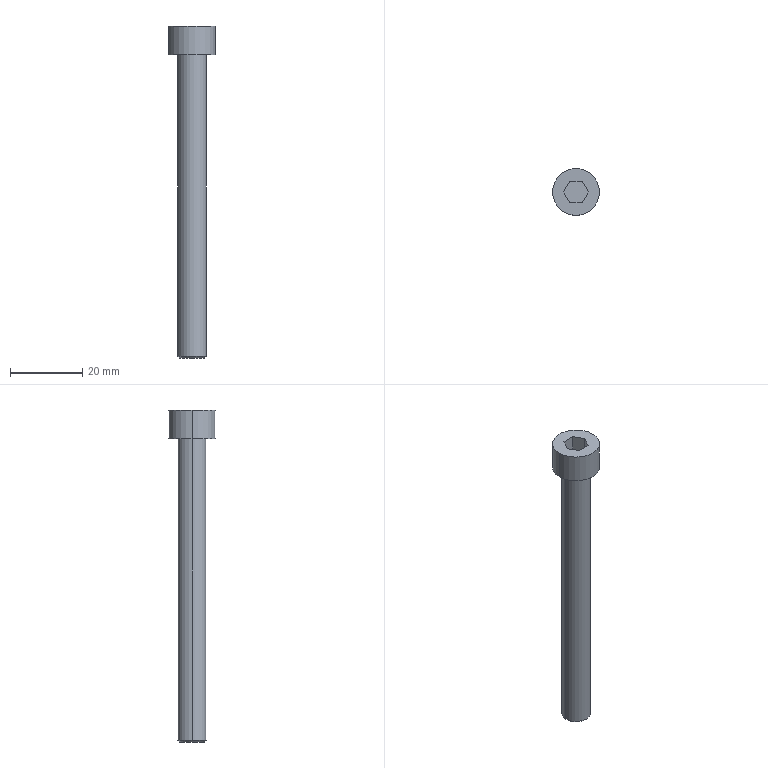Part | Creo | 1 solid | 16 faces | box 13 x 13 x 92 mm | volume 5116 mm3 | plane 10 | cylinder 4 | cone 2 | commonest cylinder face diameters 8 x2 13 x2
STEP:
#1=CARTESIAN_POINT('',(0.,0.,0.));
#2=DIRECTION('',(0.,0.,1.));
#3=DIRECTION('',(1.,0.,0.));
#4=AXIS2_PLACEMENT_3D('',#1,#2,#3);
#5=CARTESIAN_POINT('',(464.154,190.125,-122.934));
#6=VERTEX_POINT('',#5);
#7=CARTESIAN_POINT('',(472.154,190.125,-122.934));
#8=VERTEX_POINT('',#7);
#9=CARTESIAN_POINT('',(468.154,190.125,-122.934));
#10=DIRECTION('',(0.,0.,-1.));
#11=DIRECTION('',(-1.,0.,0.));
#12=AXIS2_PLACEMENT_3D('',#9,#10,#11);
#13=CIRCLE('',#12,4.);
#14=EDGE_CURVE('',#6,#8,#13,.T.);
#15=ORIENTED_EDGE('',*,*,#14,.T.);
#16=CARTESIAN_POINT('',(472.154,190.125,-39.441));
#17=VERTEX_POINT('',#16);
#18=CARTESIAN_POINT('',(472.154,190.125,-39.441));
#19=DIRECTION('',(0.,0.,-1.));
#20=VECTOR('',#19,83.493);
#21=LINE('',#18,#20);
#22=EDGE_CURVE('',#17,#8,#21,.T.);
#23=ORIENTED_EDGE('',*,*,#22,.F.);
#24=CARTESIAN_POINT('',(464.154,190.125,-39.441));
#25=VERTEX_POINT('',#24);
#26=CARTESIAN_POINT('',(468.154,190.125,-39.441));
#27=DIRECTION('',(0.,0.,1.));
#28=DIRECTION('',(1.,0.,0.));
#29=AXIS2_PLACEMENT_3D('',#26,#27,#28);
#30=CIRCLE('',#29,4.);
#31=EDGE_CURVE('',#17,#25,#30,.T.);
#32=ORIENTED_EDGE('',*,*,#31,.T.);
#33=CARTESIAN_POINT('',(464.154,190.125,-39.441));
#34=DIRECTION('',(0.,0.,-1.));
#35=VECTOR('',#34,83.493);
#36=LINE('',#33,#35);
#37=EDGE_CURVE('',#25,#6,#36,.T.);
#38=ORIENTED_EDGE('',*,*,#37,.T.);
#39=EDGE_LOOP('',(#15,#23,#32,#38));
#40=FACE_OUTER_BOUND('',#39,.F.);
#41=CARTESIAN_POINT('',(468.154,190.125,-39.441));
#42=DIRECTION('',(0.,0.,-1.));
#43=DIRECTION('',(-1.,0.,0.));
#44=AXIS2_PLACEMENT_3D('',#41,#42,#43);
#45=CYLINDRICAL_SURFACE('',#44,4.);
#46=ADVANCED_FACE('',(#40),#45,.T.);
#47=CARTESIAN_POINT('',(464.662,190.125,-123.441));
#48=VERTEX_POINT('',#47);
#49=CARTESIAN_POINT('',(471.647,190.125,-123.441));
#50=VERTEX_POINT('',#49);
#51=CARTESIAN_POINT('',(468.154,190.125,-123.441));
#52=DIRECTION('',(0.,0.,-1.));
#53=DIRECTION('',(-1.,0.,0.));
#54=AXIS2_PLACEMENT_3D('',#51,#52,#53);
#55=CIRCLE('',#54,3.493);
#56=EDGE_CURVE('',#48,#50,#55,.T.);
#57=ORIENTED_EDGE('',*,*,#56,.T.);
#58=CARTESIAN_POINT('',(471.647,190.125,-123.441));
#59=DIRECTION('',(0.7071,0.,0.7071));
#60=VECTOR('',#59,0.7176);
#61=LINE('',#58,#60);
#62=EDGE_CURVE('',#50,#8,#61,.T.);
#63=ORIENTED_EDGE('',*,*,#62,.T.);
#64=ORIENTED_EDGE('',*,*,#14,.F.);
#65=CARTESIAN_POINT('',(464.662,190.125,-123.441));
#66=DIRECTION('',(-0.7071,0.,0.7071));
#67=VECTOR('',#66,0.7176);
#68=LINE('',#65,#67);
#69=EDGE_CURVE('',#48,#6,#68,.T.);
#70=ORIENTED_EDGE('',*,*,#69,.F.);
#71=EDGE_LOOP('',(#57,#63,#64,#70));
#72=FACE_OUTER_BOUND('',#71,.F.);
#73=CARTESIAN_POINT('',(468.154,190.125,-123.188));
#74=DIRECTION('',(0.,0.,1.));
#75=DIRECTION('',(1.,0.,0.));
#76=AXIS2_PLACEMENT_3D('',#73,#74,#75);
#77=CONICAL_SURFACE('',#76,3.746,45.);
#78=ADVANCED_FACE('',(#72),#77,.T.);
#79=ORIENTED_EDGE('',*,*,#56,.F.);
#80=CARTESIAN_POINT('',(468.154,190.125,-123.441));
#81=DIRECTION('',(0.,0.,-1.));
#82=DIRECTION('',(1.,0.,0.));
#83=AXIS2_PLACEMENT_3D('',#80,#81,#82);
#84=CIRCLE('',#83,3.493);
#85=EDGE_CURVE('',#50,#48,#84,.T.);
#86=ORIENTED_EDGE('',*,*,#85,.F.);
#87=EDGE_LOOP('',(#79,#86));
#88=FACE_OUTER_BOUND('',#87,.F.);
#89=CARTESIAN_POINT('',(468.154,190.125,-123.441));
#90=DIRECTION('',(0.,0.,1.));
#91=DIRECTION('',(1.,0.,0.));
#92=AXIS2_PLACEMENT_3D('',#89,#90,#91);
#93=PLANE('',#92);
#94=ADVANCED_FACE('',(#88),#93,.F.);
#95=ORIENTED_EDGE('',*,*,#85,.T.);
#96=ORIENTED_EDGE('',*,*,#69,.T.);
#97=CARTESIAN_POINT('',(468.154,190.125,-122.934));
#98=DIRECTION('',(0.,0.,-1.));
#99=DIRECTION('',(1.,0.,0.));
#100=AXIS2_PLACEMENT_3D('',#97,#98,#99);
#101=CIRCLE('',#100,4.);
#102=EDGE_CURVE('',#8,#6,#101,.T.);
#103=ORIENTED_EDGE('',*,*,#102,.F.);
#104=ORIENTED_EDGE('',*,*,#62,.F.);
#105=EDGE_LOOP('',(#95,#96,#103,#104));
#106=FACE_OUTER_BOUND('',#105,.F.);
#107=CARTESIAN_POINT('',(468.154,190.125,-123.188));
#108=DIRECTION('',(0.,0.,1.));
#109=DIRECTION('',(1.,0.,0.));
#110=AXIS2_PLACEMENT_3D('',#107,#108,#109);
#111=CONICAL_SURFACE('',#110,3.746,45.);
#112=ADVANCED_FACE('',(#106),#111,.T.);
#113=ORIENTED_EDGE('',*,*,#102,.T.);
#114=ORIENTED_EDGE('',*,*,#37,.F.);
#115=CARTESIAN_POINT('',(468.154,190.125,-39.441));
#116=DIRECTION('',(0.,0.,1.));
#117=DIRECTION('',(-1.,0.,0.));
#118=AXIS2_PLACEMENT_3D('',#115,#116,#117);
#119=CIRCLE('',#118,4.);
#120=EDGE_CURVE('',#25,#17,#119,.T.);
#121=ORIENTED_EDGE('',*,*,#120,.T.);
#122=ORIENTED_EDGE('',*,*,#22,.T.);
#123=EDGE_LOOP('',(#113,#114,#121,#122));
#124=FACE_OUTER_BOUND('',#123,.F.);
#125=CARTESIAN_POINT('',(468.154,190.125,-39.441));
#126=DIRECTION('',(0.,0.,-1.));
#127=DIRECTION('',(-1.,0.,0.));
#128=AXIS2_PLACEMENT_3D('',#125,#126,#127);
#129=CYLINDRICAL_SURFACE('',#128,4.);
#130=ADVANCED_FACE('',(#124),#129,.T.);
#131=CARTESIAN_POINT('',(461.654,190.125,-39.441));
#132=VERTEX_POINT('',#131);
#133=CARTESIAN_POINT('',(474.654,190.125,-39.441));
#134=VERTEX_POINT('',#133);
#135=CARTESIAN_POINT('',(468.154,190.125,-39.441));
#136=DIRECTION('',(0.,0.,-1.));
#137=DIRECTION('',(-1.,0.,0.));
#138=AXIS2_PLACEMENT_3D('',#135,#136,#137);
#139=CIRCLE('',#138,6.5);
#140=EDGE_CURVE('',#132,#134,#139,.T.);
#141=ORIENTED_EDGE('',*,*,#140,.F.);
#142=CARTESIAN_POINT('',(468.154,190.125,-39.441));
#143=DIRECTION('',(0.,0.,-1.));
#144=DIRECTION('',(1.,0.,0.));
#145=AXIS2_PLACEMENT_3D('',#142,#143,#144);
#146=CIRCLE('',#145,6.5);
#147=EDGE_CURVE('',#134,#132,#146,.T.);
#148=ORIENTED_EDGE('',*,*,#147,.F.);
#149=EDGE_LOOP('',(#141,#148));
#150=FACE_OUTER_BOUND('',#149,.F.);
#151=ORIENTED_EDGE('',*,*,#120,.F.);
#152=ORIENTED_EDGE('',*,*,#31,.F.);
#153=EDGE_LOOP('',(#151,#152));
#154=FACE_BOUND('',#153,.F.);
#155=CARTESIAN_POINT('',(468.154,190.125,-39.441));
#156=DIRECTION('',(0.,0.,-1.));
#157=DIRECTION('',(-1.,0.,0.));
#158=AXIS2_PLACEMENT_3D('',#155,#156,#157);
#159=PLANE('',#158);
#160=ADVANCED_FACE('',(#150,#154),#159,.T.);
#161=CARTESIAN_POINT('',(474.654,190.125,-31.441));
#162=VERTEX_POINT('',#161);
#163=CARTESIAN_POINT('',(461.654,190.125,-31.441));
#164=VERTEX_POINT('',#163);
#165=CARTESIAN_POINT('',(468.154,190.125,-31.441));
#166=DIRECTION('',(0.,0.,1.));
#167=DIRECTION('',(1.,0.,0.));
#168=AXIS2_PLACEMENT_3D('',#165,#166,#167);
#169=CIRCLE('',#168,6.5);
#170=EDGE_CURVE('',#162,#164,#169,.T.);
#171=ORIENTED_EDGE('',*,*,#170,.T.);
#172=CARTESIAN_POINT('',(461.654,190.125,-39.441));
#173=DIRECTION('',(0.,0.,1.));
#174=VECTOR('',#173,8.);
#175=LINE('',#172,#174);
#176=EDGE_CURVE('',#132,#164,#175,.T.);
#177=ORIENTED_EDGE('',*,*,#176,.F.);
#178=ORIENTED_EDGE('',*,*,#140,.T.);
#179=CARTESIAN_POINT('',(474.654,190.125,-39.441));
#180=DIRECTION('',(0.,0.,1.));
#181=VECTOR('',#180,8.);
#182=LINE('',#179,#181);
#183=EDGE_CURVE('',#134,#162,#182,.T.);
#184=ORIENTED_EDGE('',*,*,#183,.T.);
#185=EDGE_LOOP('',(#171,#177,#178,#184));
#186=FACE_OUTER_BOUND('',#185,.F.);
#187=CARTESIAN_POINT('',(468.154,190.125,-39.441));
#188=DIRECTION('',(0.,0.,1.));
#189=DIRECTION('',(1.,0.,0.));
#190=AXIS2_PLACEMENT_3D('',#187,#188,#189);
#191=CYLINDRICAL_SURFACE('',#190,6.5);
#192=ADVANCED_FACE('',(#186),#191,.T.);
#193=CARTESIAN_POINT('',(468.154,190.125,-31.441));
#194=DIRECTION('',(0.,0.,1.));
#195=DIRECTION('',(-1.,0.,0.));
#196=AXIS2_PLACEMENT_3D('',#193,#194,#195);
#197=CIRCLE('',#196,6.5);
#198=EDGE_CURVE('',#164,#162,#197,.T.);
#199=ORIENTED_EDGE('',*,*,#198,.F.);
#200=ORIENTED_EDGE('',*,*,#170,.F.);
#201=EDGE_LOOP('',(#199,#200));
#202=FACE_OUTER_BOUND('',#201,.F.);
#203=CARTESIAN_POINT('',(466.422,193.125,-31.441));
#204=VERTEX_POINT('',#203);
#205=CARTESIAN_POINT('',(469.886,193.125,-31.441));
#206=VERTEX_POINT('',#205);
#207=CARTESIAN_POINT('',(466.422,193.125,-31.441));
#208=DIRECTION('',(1.,0.,0.));
#209=VECTOR('',#208,3.464);
#210=LINE('',#207,#209);
#211=EDGE_CURVE('',#204,#206,#210,.T.);
#212=ORIENTED_EDGE('',*,*,#211,.F.);
#213=CARTESIAN_POINT('',(464.69,190.125,-31.441));
#214=VERTEX_POINT('',#213);
#215=CARTESIAN_POINT('',(464.69,190.125,-31.441));
#216=DIRECTION('',(0.5,0.866,0.));
#217=VECTOR('',#216,3.464);
#218=LINE('',#215,#217);
#219=EDGE_CURVE('',#214,#204,#218,.T.);
#220=ORIENTED_EDGE('',*,*,#219,.F.);
#221=CARTESIAN_POINT('',(466.422,187.125,-31.441));
#222=VERTEX_POINT('',#221);
#223=CARTESIAN_POINT('',(466.422,187.125,-31.441));
#224=DIRECTION('',(-0.5,0.866,0.));
#225=VECTOR('',#224,3.464);
#226=LINE('',#223,#225);
#227=EDGE_CURVE('',#222,#214,#226,.T.);
#228=ORIENTED_EDGE('',*,*,#227,.F.);
#229=CARTESIAN_POINT('',(469.886,187.125,-31.441));
#230=VERTEX_POINT('',#229);
#231=CARTESIAN_POINT('',(469.886,187.125,-31.441));
#232=DIRECTION('',(-1.,0.,0.));
#233=VECTOR('',#232,3.464);
#234=LINE('',#231,#233);
#235=EDGE_CURVE('',#230,#222,#234,.T.);
#236=ORIENTED_EDGE('',*,*,#235,.F.);
#237=CARTESIAN_POINT('',(471.618,190.125,-31.441));
#238=VERTEX_POINT('',#237);
#239=CARTESIAN_POINT('',(471.618,190.125,-31.441));
#240=DIRECTION('',(-0.5,-0.866,0.));
#241=VECTOR('',#240,3.464);
#242=LINE('',#239,#241);
#243=EDGE_CURVE('',#238,#230,#242,.T.);
#244=ORIENTED_EDGE('',*,*,#243,.F.);
#245=CARTESIAN_POINT('',(469.886,193.125,-31.441));
#246=DIRECTION('',(0.5,-0.866,0.));
#247=VECTOR('',#246,3.464);
#248=LINE('',#245,#247);
#249=EDGE_CURVE('',#206,#238,#248,.T.);
#250=ORIENTED_EDGE('',*,*,#249,.F.);
#251=EDGE_LOOP('',(#212,#220,#228,#236,#244,#250));
#252=FACE_BOUND('',#251,.F.);
#253=CARTESIAN_POINT('',(468.154,190.125,-31.441));
#254=DIRECTION('',(0.,0.,1.));
#255=DIRECTION('',(1.,0.,0.));
#256=AXIS2_PLACEMENT_3D('',#253,#254,#255);
#257=PLANE('',#256);
#258=ADVANCED_FACE('',(#202,#252),#257,.T.);
#259=ORIENTED_EDGE('',*,*,#211,.T.);
#260=CARTESIAN_POINT('',(469.886,193.125,-36.721));
#261=VERTEX_POINT('',#260);
#262=CARTESIAN_POINT('',(469.886,193.125,-31.441));
#263=DIRECTION('',(0.,0.,-1.));
#264=VECTOR('',#263,5.28);
#265=LINE('',#262,#264);
#266=EDGE_CURVE('',#206,#261,#265,.T.);
#267=ORIENTED_EDGE('',*,*,#266,.T.);
#268=CARTESIAN_POINT('',(466.422,193.125,-36.721));
#269=VERTEX_POINT('',#268);
#270=CARTESIAN_POINT('',(466.422,193.125,-36.721));
#271=DIRECTION('',(1.,0.,0.));
#272=VECTOR('',#271,3.464);
#273=LINE('',#270,#272);
#274=EDGE_CURVE('',#269,#261,#273,.T.);
#275=ORIENTED_EDGE('',*,*,#274,.F.);
#276=CARTESIAN_POINT('',(466.422,193.125,-31.441));
#277=DIRECTION('',(0.,0.,-1.));
#278=VECTOR('',#277,5.28);
#279=LINE('',#276,#278);
#280=EDGE_CURVE('',#204,#269,#279,.T.);
#281=ORIENTED_EDGE('',*,*,#280,.F.);
#282=EDGE_LOOP('',(#259,#267,#275,#281));
#283=FACE_OUTER_BOUND('',#282,.F.);
#284=CARTESIAN_POINT('',(469.886,193.125,-36.721));
#285=DIRECTION('',(0.,1.,0.));
#286=DIRECTION('',(0.,0.,1.));
#287=AXIS2_PLACEMENT_3D('',#284,#285,#286);
#288=PLANE('',#287);
#289=ADVANCED_FACE('',(#283),#288,.F.);
#290=ORIENTED_EDGE('',*,*,#249,.T.);
#291=CARTESIAN_POINT('',(471.618,190.125,-36.721));
#292=VERTEX_POINT('',#291);
#293=CARTESIAN_POINT('',(471.618,190.125,-31.441));
#294=DIRECTION('',(0.,0.,-1.));
#295=VECTOR('',#294,5.28);
#296=LINE('',#293,#295);
#297=EDGE_CURVE('',#238,#292,#296,.T.);
#298=ORIENTED_EDGE('',*,*,#297,.T.);
#299=CARTESIAN_POINT('',(471.618,190.125,-36.721));
#300=DIRECTION('',(-0.5,0.866,0.));
#301=VECTOR('',#300,3.464);
#302=LINE('',#299,#301);
#303=EDGE_CURVE('',#292,#261,#302,.T.);
#304=ORIENTED_EDGE('',*,*,#303,.T.);
#305=ORIENTED_EDGE('',*,*,#266,.F.);
#306=EDGE_LOOP('',(#290,#298,#304,#305));
#307=FACE_OUTER_BOUND('',#306,.F.);
#308=CARTESIAN_POINT('',(471.618,190.125,-36.721));
#309=DIRECTION('',(0.866,0.5,0.));
#310=DIRECTION('',(-0.5,0.866,0.));
#311=AXIS2_PLACEMENT_3D('',#308,#309,#310);
#312=PLANE('',#311);
#313=ADVANCED_FACE('',(#307),#312,.F.);
#314=ORIENTED_EDGE('',*,*,#243,.T.);
#315=CARTESIAN_POINT('',(469.886,187.125,-36.721));
#316=VERTEX_POINT('',#315);
#317=CARTESIAN_POINT('',(469.886,187.125,-31.441));
#318=DIRECTION('',(0.,0.,-1.));
#319=VECTOR('',#318,5.28);
#320=LINE('',#317,#319);
#321=EDGE_CURVE('',#230,#316,#320,.T.);
#322=ORIENTED_EDGE('',*,*,#321,.T.);
#323=CARTESIAN_POINT('',(469.886,187.125,-36.721));
#324=DIRECTION('',(0.5,0.866,0.));
#325=VECTOR('',#324,3.464);
#326=LINE('',#323,#325);
#327=EDGE_CURVE('',#316,#292,#326,.T.);
#328=ORIENTED_EDGE('',*,*,#327,.T.);
#329=ORIENTED_EDGE('',*,*,#297,.F.);
#330=EDGE_LOOP('',(#314,#322,#328,#329));
#331=FACE_OUTER_BOUND('',#330,.F.);
#332=CARTESIAN_POINT('',(469.886,187.125,-36.721));
#333=DIRECTION('',(0.866,-0.5,0.));
#334=DIRECTION('',(0.5,0.866,0.));
#335=AXIS2_PLACEMENT_3D('',#332,#333,#334);
#336=PLANE('',#335);
#337=ADVANCED_FACE('',(#331),#336,.F.);
#338=ORIENTED_EDGE('',*,*,#235,.T.);
#339=CARTESIAN_POINT('',(466.422,187.125,-36.721));
#340=VERTEX_POINT('',#339);
#341=CARTESIAN_POINT('',(466.422,187.125,-31.441));
#342=DIRECTION('',(0.,0.,-1.));
#343=VECTOR('',#342,5.28);
#344=LINE('',#341,#343);
#345=EDGE_CURVE('',#222,#340,#344,.T.);
#346=ORIENTED_EDGE('',*,*,#345,.T.);
#347=CARTESIAN_POINT('',(469.886,187.125,-36.721));
#348=DIRECTION('',(-1.,0.,0.));
#349=VECTOR('',#348,3.464);
#350=LINE('',#347,#349);
#351=EDGE_CURVE('',#316,#340,#350,.T.);
#352=ORIENTED_EDGE('',*,*,#351,.F.);
#353=ORIENTED_EDGE('',*,*,#321,.F.);
#354=EDGE_LOOP('',(#338,#346,#352,#353));
#355=FACE_OUTER_BOUND('',#354,.F.);
#356=CARTESIAN_POINT('',(466.422,187.125,-36.721));
#357=DIRECTION('',(0.,-1.,0.));
#358=DIRECTION('',(0.,0.,-1.));
#359=AXIS2_PLACEMENT_3D('',#356,#357,#358);
#360=PLANE('',#359);
#361=ADVANCED_FACE('',(#355),#360,.F.);
#362=ORIENTED_EDGE('',*,*,#227,.T.);
#363=CARTESIAN_POINT('',(464.69,190.125,-36.721));
#364=VERTEX_POINT('',#363);
#365=CARTESIAN_POINT('',(464.69,190.125,-31.441));
#366=DIRECTION('',(0.,0.,-1.));
#367=VECTOR('',#366,5.28);
#368=LINE('',#365,#367);
#369=EDGE_CURVE('',#214,#364,#368,.T.);
#370=ORIENTED_EDGE('',*,*,#369,.T.);
#371=CARTESIAN_POINT('',(464.69,190.125,-36.721));
#372=DIRECTION('',(0.5,-0.866,0.));
#373=VECTOR('',#372,3.464);
#374=LINE('',#371,#373);
#375=EDGE_CURVE('',#364,#340,#374,.T.);
#376=ORIENTED_EDGE('',*,*,#375,.T.);
#377=ORIENTED_EDGE('',*,*,#345,.F.);
#378=EDGE_LOOP('',(#362,#370,#376,#377));
#379=FACE_OUTER_BOUND('',#378,.F.);
#380=CARTESIAN_POINT('',(464.69,190.125,-36.721));
#381=DIRECTION('',(-0.866,-0.5,0.));
#382=DIRECTION('',(0.5,-0.866,0.));
#383=AXIS2_PLACEMENT_3D('',#380,#381,#382);
#384=PLANE('',#383);
#385=ADVANCED_FACE('',(#379),#384,.F.);
#386=ORIENTED_EDGE('',*,*,#219,.T.);
#387=ORIENTED_EDGE('',*,*,#280,.T.);
#388=CARTESIAN_POINT('',(466.422,193.125,-36.721));
#389=DIRECTION('',(-0.5,-0.866,0.));
#390=VECTOR('',#389,3.464);
#391=LINE('',#388,#390);
#392=EDGE_CURVE('',#269,#364,#391,.T.);
#393=ORIENTED_EDGE('',*,*,#392,.T.);
#394=ORIENTED_EDGE('',*,*,#369,.F.);
#395=EDGE_LOOP('',(#386,#387,#393,#394));
#396=FACE_OUTER_BOUND('',#395,.F.);
#397=CARTESIAN_POINT('',(466.422,193.125,-36.721));
#398=DIRECTION('',(-0.866,0.5,0.));
#399=DIRECTION('',(-0.5,-0.866,0.));
#400=AXIS2_PLACEMENT_3D('',#397,#398,#399);
#401=PLANE('',#400);
#402=ADVANCED_FACE('',(#396),#401,.F.);
#403=ORIENTED_EDGE('',*,*,#274,.T.);
#404=ORIENTED_EDGE('',*,*,#303,.F.);
#405=ORIENTED_EDGE('',*,*,#327,.F.);
#406=ORIENTED_EDGE('',*,*,#351,.T.);
#407=ORIENTED_EDGE('',*,*,#375,.F.);
#408=ORIENTED_EDGE('',*,*,#392,.F.);
#409=EDGE_LOOP('',(#403,#404,#405,#406,#407,#408));
#410=FACE_OUTER_BOUND('',#409,.F.);
#411=CARTESIAN_POINT('',(466.422,193.125,-36.721));
#412=DIRECTION('',(0.,0.,1.));
#413=DIRECTION('',(1.,0.,0.));
#414=AXIS2_PLACEMENT_3D('',#411,#412,#413);
#415=PLANE('',#414);
#416=ADVANCED_FACE('',(#410),#415,.T.);
#417=ORIENTED_EDGE('',*,*,#198,.T.);
#418=ORIENTED_EDGE('',*,*,#183,.F.);
#419=ORIENTED_EDGE('',*,*,#147,.T.);
#420=ORIENTED_EDGE('',*,*,#176,.T.);
#421=EDGE_LOOP('',(#417,#418,#419,#420));
#422=FACE_OUTER_BOUND('',#421,.F.);
#423=CARTESIAN_POINT('',(468.154,190.125,-39.441));
#424=DIRECTION('',(0.,0.,1.));
#425=DIRECTION('',(1.,0.,0.));
#426=AXIS2_PLACEMENT_3D('',#423,#424,#425);
#427=CYLINDRICAL_SURFACE('',#426,6.5);
#428=ADVANCED_FACE('',(#422),#427,.T.);
#429=CLOSED_SHELL('',(#46,#78,#94,#112,#130,#160,#192,#258,#289,#313,#337,#361,#385,#402,#416,#428));
#430=MANIFOLD_SOLID_BREP('',#429);
#431=(LENGTH_UNIT()NAMED_UNIT(*)SI_UNIT(.MILLI.,.METRE.));
#432=UNCERTAINTY_MEASURE_WITH_UNIT(LENGTH_MEASURE(0.009382),#431,'','');
#433=(NAMED_UNIT(*)PLANE_ANGLE_UNIT()SI_UNIT($,.RADIAN.));
#434=PLANE_ANGLE_MEASURE_WITH_UNIT(PLANE_ANGLE_MEASURE(0.01745),#433);
#435=(CONVERSION_BASED_UNIT('DEGREE',#434)NAMED_UNIT(*)PLANE_ANGLE_UNIT());
#436=(NAMED_UNIT(*)SI_UNIT($,.STERADIAN.)SOLID_ANGLE_UNIT());
#437=(GEOMETRIC_REPRESENTATION_CONTEXT(3)GLOBAL_UNCERTAINTY_ASSIGNED_CONTEXT((#432))GLOBAL_UNIT_ASSIGNED_CONTEXT((#431,#435,#436))REPRESENTATION_CONTEXT('',''));
#438=ADVANCED_BREP_SHAPE_REPRESENTATION('',(#4,#430),#437);